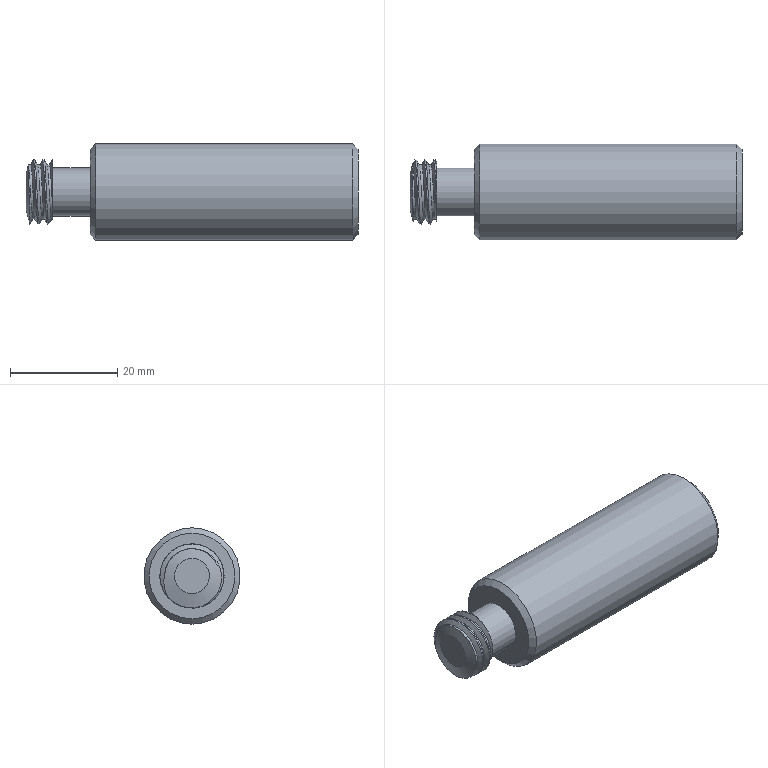Part | NX | features DATUM_CSYS 2, CHAMFER 1, SKETCH 1, SWP104 1, THREADS 1 | 1 solid | 13 faces | box 62 x 18 x 18 mm | volume 13574 mm3 | cylinder 4 | plane 4 | spline 2 | cone 2 | sphere 1 | commonest cylinder face diameters 9 x1 10.25 x1 12 x1 18 x1
STEP:
#1=CARTESIAN_POINT('',(-57.,-2.651,5.382));
#2=VERTEX_POINT('',#1);
#3=CARTESIAN_POINT('',(-57.,2.651,5.382));
#4=VERTEX_POINT('',#3);
#5=CARTESIAN_POINT('',(-57.,0.,0.));
#6=DIRECTION('',(-1.,0.,0.));
#7=DIRECTION('',(0.,0.,1.));
#8=AXIS2_PLACEMENT_3D('',#5,#6,#7);
#9=CIRCLE('',#8,6.);
#10=EDGE_CURVE('',#2,#4,#9,.T.);
#11=ORIENTED_EDGE('',*,*,#10,.T.);
#12=CARTESIAN_POINT('',(-61.271,-0.4952,-5.98));
#13=VERTEX_POINT('',#12);
#14=CARTESIAN_POINT('',(-57.,2.651,5.382));
#15=CARTESIAN_POINT('',(-57.09,4.387,4.527));
#16=CARTESIAN_POINT('',(-57.266,6.894,1.087));
#17=CARTESIAN_POINT('',(-57.534,4.858,-5.032));
#18=CARTESIAN_POINT('',(-57.801,-1.327,-6.864));
#19=CARTESIAN_POINT('',(-58.067,-6.379,-2.86));
#20=CARTESIAN_POINT('',(-58.335,-6.007,3.575));
#21=CARTESIAN_POINT('',(-58.601,-0.5304,6.969));
#22=CARTESIAN_POINT('',(-58.868,5.395,4.444));
#23=CARTESIAN_POINT('',(-59.135,6.739,-1.86));
#24=CARTESIAN_POINT('',(-59.402,2.351,-6.584));
#25=CARTESIAN_POINT('',(-59.669,-4.036,-5.708));
#26=CARTESIAN_POINT('',(-59.936,-6.99,0.02189));
#27=CARTESIAN_POINT('',(-60.203,-4.002,5.73));
#28=CARTESIAN_POINT('',(-60.469,2.383,6.571));
#29=CARTESIAN_POINT('',(-60.736,6.75,1.827));
#30=CARTESIAN_POINT('',(-61.004,5.364,-4.47));
#31=CARTESIAN_POINT('',(-61.18,1.433,-6.139));
#32=CARTESIAN_POINT('',(-61.271,-0.4952,-5.98));
#33=B_SPLINE_CURVE_WITH_KNOTS('',3,(#14,#15,#16,#17,#18,#19,#20,#21,#22,#23,#24,#25,#26,#27,#28,#29,#30,#31,#32),.UNSPECIFIED.,.F.,.F.,(4,1,1,1,1,1,1,1,1,1,1,1,1,1,1,1,4),(0.,0.005728,0.01146,0.01719,0.02291,0.02864,0.03437,0.0401,0.04583,0.05156,0.05728,0.06301,0.06874,0.07447,0.0802,0.08593,0.09165),.UNSPECIFIED.);
#34=EDGE_CURVE('',#4,#13,#33,.T.);
#35=ORIENTED_EDGE('',*,*,#34,.T.);
#36=CARTESIAN_POINT('',(-61.271,4.439,-4.037));
#37=VERTEX_POINT('',#36);
#38=CARTESIAN_POINT('',(-61.271,0.,0.));
#39=DIRECTION('',(-1.,0.,0.));
#40=DIRECTION('',(0.,0.,1.));
#41=AXIS2_PLACEMENT_3D('',#38,#39,#40);
#42=CIRCLE('',#41,6.);
#43=EDGE_CURVE('',#37,#13,#42,.T.);
#44=ORIENTED_EDGE('',*,*,#43,.F.);
#45=CARTESIAN_POINT('',(-61.271,4.439,-4.037));
#46=CARTESIAN_POINT('',(-61.18,5.741,-2.606));
#47=CARTESIAN_POINT('',(-61.004,6.813,1.514));
#48=CARTESIAN_POINT('',(-60.737,2.677,6.462));
#49=CARTESIAN_POINT('',(-60.47,-3.749,5.901));
#50=CARTESIAN_POINT('',(-60.203,-6.983,0.3245));
#51=CARTESIAN_POINT('',(-59.936,-4.279,-5.527));
#52=CARTESIAN_POINT('',(-59.669,2.06,-6.679));
#53=CARTESIAN_POINT('',(-59.402,6.648,-2.158));
#54=CARTESIAN_POINT('',(-59.135,5.589,4.199));
#55=CARTESIAN_POINT('',(-58.869,-0.2242,6.987));
#56=CARTESIAN_POINT('',(-58.601,-5.847,3.832));
#57=CARTESIAN_POINT('',(-58.335,-6.496,-2.581));
#58=CARTESIAN_POINT('',(-58.068,-1.624,-6.798));
#59=CARTESIAN_POINT('',(-57.801,4.625,-5.241));
#60=CARTESIAN_POINT('',(-57.534,6.95,0.7729));
#61=CARTESIAN_POINT('',(-57.267,3.353,6.124));
#62=CARTESIAN_POINT('',(-57.09,-0.9155,6.237));
#63=CARTESIAN_POINT('',(-57.,-2.651,5.382));
#64=B_SPLINE_CURVE_WITH_KNOTS('',3,(#45,#46,#47,#48,#49,#50,#51,#52,#53,#54,#55,#56,#57,#58,#59,#60,#61,#62,#63),.UNSPECIFIED.,.F.,.F.,(4,1,1,1,1,1,1,1,1,1,1,1,1,1,1,1,4),(0.,0.005728,0.01146,0.01719,0.02291,0.02864,0.03437,0.0401,0.04583,0.05156,0.05728,0.06301,0.06874,0.07447,0.0802,0.08593,0.09165),.UNSPECIFIED.);
#65=EDGE_CURVE('',#37,#2,#64,.T.);
#66=ORIENTED_EDGE('',*,*,#65,.T.);
#67=EDGE_LOOP('',(#11,#35,#44,#66));
#68=FACE_BOUND('',#67,.T.);
#69=CARTESIAN_POINT('',(0.,0.,0.));
#70=DIRECTION('',(-1.,0.,0.));
#71=DIRECTION('',(0.,0.,1.));
#72=AXIS2_PLACEMENT_3D('',#69,#70,#71);
#73=CYLINDRICAL_SURFACE('',#72,6.);
#74=ADVANCED_FACE('',(#68),#73,.T.);
#75=CARTESIAN_POINT('',(-62.,0.,3.273));
#76=VERTEX_POINT('',#75);
#77=CARTESIAN_POINT('',(-62.,0.,0.));
#78=DIRECTION('',(-1.,0.,0.));
#79=DIRECTION('',(0.,0.,1.));
#80=AXIS2_PLACEMENT_3D('',#77,#78,#79);
#81=CIRCLE('',#80,3.273);
#82=EDGE_CURVE('',#76,#76,#81,.T.);
#83=ORIENTED_EDGE('',*,*,#82,.F.);
#84=EDGE_LOOP('',(#83));
#85=FACE_BOUND('',#84,.T.);
#86=ORIENTED_EDGE('',*,*,#43,.T.);
#87=CARTESIAN_POINT('',(-61.555,-1.14,4.997));
#88=VERTEX_POINT('',#87);
#89=CARTESIAN_POINT('',(-61.271,-0.4952,-5.98));
#90=CARTESIAN_POINT('',(-61.294,-1.812,-5.804));
#91=CARTESIAN_POINT('',(-61.34,-4.284,-4.566));
#92=CARTESIAN_POINT('',(-61.411,-6.03,-0.7463));
#93=CARTESIAN_POINT('',(-61.483,-4.847,3.306));
#94=CARTESIAN_POINT('',(-61.53,-2.452,4.782));
#95=CARTESIAN_POINT('',(-61.555,-1.14,4.997));
#96=B_SPLINE_CURVE_WITH_KNOTS('',3,(#89,#90,#91,#92,#93,#94,#95),.UNSPECIFIED.,.F.,.F.,(4,1,1,1,4),(0.,0.003931,0.007861,0.01179,0.01572),.UNSPECIFIED.);
#97=EDGE_CURVE('',#13,#88,#96,.T.);
#98=ORIENTED_EDGE('',*,*,#97,.T.);
#99=CARTESIAN_POINT('',(-61.555,5.117,0.2797));
#100=VERTEX_POINT('',#99);
#101=CARTESIAN_POINT('',(-61.555,0.,0.));
#102=DIRECTION('',(1.,0.,0.));
#103=DIRECTION('',(0.,0.,-1.));
#104=AXIS2_PLACEMENT_3D('',#101,#102,#103);
#105=CIRCLE('',#104,5.125);
#106=EDGE_CURVE('',#100,#88,#105,.T.);
#107=ORIENTED_EDGE('',*,*,#106,.F.);
#108=CARTESIAN_POINT('',(-61.555,5.117,0.2797));
#109=CARTESIAN_POINT('',(-61.469,5.486,-1.181));
#110=CARTESIAN_POINT('',(-61.379,5.202,-2.742));
#111=CARTESIAN_POINT('',(-61.271,4.439,-4.037));
#112=B_SPLINE_CURVE_WITH_KNOTS('',3,(#108,#109,#110,#111),.UNSPECIFIED.,.F.,.F.,(4,4),(0.00002886,0.004494),.UNSPECIFIED.);
#113=EDGE_CURVE('',#100,#37,#112,.T.);
#114=ORIENTED_EDGE('',*,*,#113,.T.);
#115=EDGE_LOOP('',(#86,#98,#107,#114));
#116=FACE_BOUND('',#115,.T.);
#117=CARTESIAN_POINT('',(-44.3,0.,0.));
#118=DIRECTION('',(-1.,0.,0.));
#119=DIRECTION('',(0.,1.,0.));
#120=AXIS2_PLACEMENT_3D('',#117,#118,#119);
#121=SPHERICAL_SURFACE('',#120,18.);
#122=ADVANCED_FACE('',(#85,#116),#121,.T.);
#123=ORIENTED_EDGE('',*,*,#82,.T.);
#124=EDGE_LOOP('',(#123));
#125=FACE_BOUND('',#124,.T.);
#126=CARTESIAN_POINT('',(-62.,3.273,0.));
#127=DIRECTION('',(1.,0.,0.));
#128=DIRECTION('',(0.,0.,-1.));
#129=AXIS2_PLACEMENT_3D('',#126,#127,#128);
#130=PLANE('',#129);
#131=ADVANCED_FACE('',(#125),#130,.F.);
#132=CARTESIAN_POINT('',(0.,0.,8.));
#133=VERTEX_POINT('',#132);
#134=CARTESIAN_POINT('',(0.,0.,0.));
#135=DIRECTION('',(-1.,0.,0.));
#136=DIRECTION('',(0.,0.,1.));
#137=AXIS2_PLACEMENT_3D('',#134,#135,#136);
#138=CIRCLE('',#137,8.);
#139=EDGE_CURVE('',#133,#133,#138,.F.);
#140=ORIENTED_EDGE('',*,*,#139,.T.);
#141=EDGE_LOOP('',(#140));
#142=FACE_BOUND('',#141,.T.);
#143=CARTESIAN_POINT('',(0.,0.,0.));
#144=DIRECTION('',(-1.,0.,0.));
#145=DIRECTION('',(0.,0.,1.));
#146=AXIS2_PLACEMENT_3D('',#143,#144,#145);
#147=PLANE('',#146);
#148=ADVANCED_FACE('',(#142),#147,.F.);
#149=CARTESIAN_POINT('',(-49.,0.,-9.));
#150=VERTEX_POINT('',#149);
#151=CARTESIAN_POINT('',(-49.,0.,0.));
#152=DIRECTION('',(1.,0.,0.));
#153=DIRECTION('',(0.,0.,-1.));
#154=AXIS2_PLACEMENT_3D('',#151,#152,#153);
#155=CIRCLE('',#154,9.);
#156=EDGE_CURVE('',#150,#150,#155,.T.);
#157=ORIENTED_EDGE('',*,*,#156,.T.);
#158=EDGE_LOOP('',(#157));
#159=FACE_BOUND('',#158,.T.);
#160=CARTESIAN_POINT('',(-1.,0.,9.));
#161=VERTEX_POINT('',#160);
#162=CARTESIAN_POINT('',(-1.,0.,0.));
#163=DIRECTION('',(-1.,0.,0.));
#164=DIRECTION('',(0.,0.,1.));
#165=AXIS2_PLACEMENT_3D('',#162,#163,#164);
#166=CIRCLE('',#165,9.);
#167=EDGE_CURVE('',#161,#161,#166,.T.);
#168=ORIENTED_EDGE('',*,*,#167,.T.);
#169=EDGE_LOOP('',(#168));
#170=FACE_BOUND('',#169,.T.);
#171=CARTESIAN_POINT('',(0.,0.,0.));
#172=DIRECTION('',(-1.,0.,0.));
#173=DIRECTION('',(0.,0.,1.));
#174=AXIS2_PLACEMENT_3D('',#171,#172,#173);
#175=CYLINDRICAL_SURFACE('',#174,9.);
#176=ADVANCED_FACE('',(#159,#170),#175,.T.);
#177=CARTESIAN_POINT('',(-50.,0.,-8.));
#178=VERTEX_POINT('',#177);
#179=CARTESIAN_POINT('',(-50.,0.,0.));
#180=DIRECTION('',(1.,0.,0.));
#181=DIRECTION('',(0.,0.,-1.));
#182=AXIS2_PLACEMENT_3D('',#179,#180,#181);
#183=CIRCLE('',#182,8.);
#184=EDGE_CURVE('',#178,#178,#183,.F.);
#185=ORIENTED_EDGE('',*,*,#184,.T.);
#186=EDGE_LOOP('',(#185));
#187=FACE_BOUND('',#186,.T.);
#188=CARTESIAN_POINT('',(-50.,0.,4.5));
#189=VERTEX_POINT('',#188);
#190=CARTESIAN_POINT('',(-50.,0.,0.));
#191=DIRECTION('',(-1.,0.,0.));
#192=DIRECTION('',(0.,0.,1.));
#193=AXIS2_PLACEMENT_3D('',#190,#191,#192);
#194=CIRCLE('',#193,4.5);
#195=EDGE_CURVE('',#189,#189,#194,.T.);
#196=ORIENTED_EDGE('',*,*,#195,.F.);
#197=EDGE_LOOP('',(#196));
#198=FACE_BOUND('',#197,.T.);
#199=CARTESIAN_POINT('',(-50.,9.,0.));
#200=DIRECTION('',(1.,0.,0.));
#201=DIRECTION('',(0.,0.,-1.));
#202=AXIS2_PLACEMENT_3D('',#199,#200,#201);
#203=PLANE('',#202);
#204=ADVANCED_FACE('',(#187,#198),#203,.F.);
#205=CARTESIAN_POINT('',(-57.,0.,4.5));
#206=VERTEX_POINT('',#205);
#207=CARTESIAN_POINT('',(-57.,0.,0.));
#208=DIRECTION('',(-1.,0.,0.));
#209=DIRECTION('',(0.,0.,1.));
#210=AXIS2_PLACEMENT_3D('',#207,#208,#209);
#211=CIRCLE('',#210,4.5);
#212=EDGE_CURVE('',#206,#206,#211,.T.);
#213=ORIENTED_EDGE('',*,*,#212,.F.);
#214=EDGE_LOOP('',(#213));
#215=FACE_BOUND('',#214,.T.);
#216=ORIENTED_EDGE('',*,*,#195,.T.);
#217=EDGE_LOOP('',(#216));
#218=FACE_BOUND('',#217,.T.);
#219=CARTESIAN_POINT('',(0.,0.,0.));
#220=DIRECTION('',(-1.,0.,0.));
#221=DIRECTION('',(0.,0.,1.));
#222=AXIS2_PLACEMENT_3D('',#219,#220,#221);
#223=CYLINDRICAL_SURFACE('',#222,4.5);
#224=ADVANCED_FACE('',(#215,#218),#223,.T.);
#225=ORIENTED_EDGE('',*,*,#10,.F.);
#226=CARTESIAN_POINT('',(-57.,-3.918,-3.304));
#227=VERTEX_POINT('',#226);
#228=CARTESIAN_POINT('',(-57.,-2.651,5.382));
#229=CARTESIAN_POINT('',(-57.,-4.109,4.512));
#230=CARTESIAN_POINT('',(-57.,-6.212,1.478));
#231=CARTESIAN_POINT('',(-57.,-5.133,-2.11));
#232=CARTESIAN_POINT('',(-57.,-3.918,-3.304));
#233=B_SPLINE_CURVE_WITH_KNOTS('',3,(#228,#229,#230,#231,#232),.UNSPECIFIED.,.F.,.F.,(4,1,4),(0.0001216,0.005159,0.0102),.UNSPECIFIED.);
#234=EDGE_CURVE('',#2,#227,#233,.T.);
#235=ORIENTED_EDGE('',*,*,#234,.T.);
#236=CARTESIAN_POINT('',(-57.,3.918,-3.304));
#237=VERTEX_POINT('',#236);
#238=CARTESIAN_POINT('',(-57.,0.,0.));
#239=DIRECTION('',(-1.,0.,0.));
#240=DIRECTION('',(0.,0.,1.));
#241=AXIS2_PLACEMENT_3D('',#238,#239,#240);
#242=CIRCLE('',#241,5.125);
#243=EDGE_CURVE('',#237,#227,#242,.T.);
#244=ORIENTED_EDGE('',*,*,#243,.F.);
#245=CARTESIAN_POINT('',(-57.,3.918,-3.304));
#246=CARTESIAN_POINT('',(-57.,5.13,-2.112));
#247=CARTESIAN_POINT('',(-57.,6.216,1.465));
#248=CARTESIAN_POINT('',(-57.,4.109,4.512));
#249=CARTESIAN_POINT('',(-57.,2.651,5.382));
#250=B_SPLINE_CURVE_WITH_KNOTS('',3,(#245,#246,#247,#248,#249),.UNSPECIFIED.,.F.,.F.,(4,1,4),(0.00005946,0.005098,0.01014),.UNSPECIFIED.);
#251=EDGE_CURVE('',#237,#4,#250,.T.);
#252=ORIENTED_EDGE('',*,*,#251,.T.);
#253=EDGE_LOOP('',(#225,#235,#244,#252));
#254=FACE_BOUND('',#253,.T.);
#255=ORIENTED_EDGE('',*,*,#212,.T.);
#256=EDGE_LOOP('',(#255));
#257=FACE_BOUND('',#256,.T.);
#258=CARTESIAN_POINT('',(-57.,4.5,0.));
#259=DIRECTION('',(-1.,0.,0.));
#260=DIRECTION('',(0.,0.,1.));
#261=AXIS2_PLACEMENT_3D('',#258,#259,#260);
#262=PLANE('',#261);
#263=ADVANCED_FACE('',(#254,#257),#262,.F.);
#264=ORIENTED_EDGE('',*,*,#243,.T.);
#265=CARTESIAN_POINT('',(-61.555,5.117,0.2797));
#266=CARTESIAN_POINT('',(-61.46,5.022,2.017));
#267=CARTESIAN_POINT('',(-61.27,2.892,5.365));
#268=CARTESIAN_POINT('',(-60.985,-3.072,5.268));
#269=CARTESIAN_POINT('',(-60.701,-6.096,0.1263));
#270=CARTESIAN_POINT('',(-60.416,-3.288,-5.135));
#271=CARTESIAN_POINT('',(-60.132,2.667,-5.483));
#272=CARTESIAN_POINT('',(-59.847,6.069,-0.5848));
#273=CARTESIAN_POINT('',(-59.562,3.664,4.873));
#274=CARTESIAN_POINT('',(-59.278,-2.247,5.668));
#275=CARTESIAN_POINT('',(-58.993,-6.008,1.039));
#276=CARTESIAN_POINT('',(-58.708,-4.02,-4.584));
#277=CARTESIAN_POINT('',(-58.423,1.815,-5.821));
#278=CARTESIAN_POINT('',(-58.139,5.913,-1.487));
#279=CARTESIAN_POINT('',(-57.854,4.354,4.269));
#280=CARTESIAN_POINT('',(-57.569,-1.375,5.943));
#281=CARTESIAN_POINT('',(-57.285,-5.778,1.919));
#282=CARTESIAN_POINT('',(-57.095,-5.05,-1.961));
#283=CARTESIAN_POINT('',(-57.,-3.918,-3.304));
#284=B_SPLINE_CURVE_WITH_KNOTS('',3,(#265,#266,#267,#268,#269,#270,#271,#272,#273,#274,#275,#276,#277,#278,#279,#280,#281,#282,#283),.UNSPECIFIED.,.F.,.F.,(4,1,1,1,1,1,1,1,1,1,1,1,1,1,1,1,4),(0.009769,0.01499,0.02021,0.02543,0.03065,0.03588,0.0411,0.04632,0.05154,0.05676,0.06198,0.0672,0.07242,0.07764,0.08287,0.08809,0.09331),.UNSPECIFIED.);
#285=EDGE_CURVE('',#227,#100,#284,.F.);
#286=ORIENTED_EDGE('',*,*,#285,.T.);
#287=ORIENTED_EDGE('',*,*,#106,.T.);
#288=CARTESIAN_POINT('',(-57.,3.918,-3.304));
#289=CARTESIAN_POINT('',(-57.094,2.794,-4.636));
#290=CARTESIAN_POINT('',(-57.285,-0.9202,-6.024));
#291=CARTESIAN_POINT('',(-57.569,-5.624,-2.357));
#292=CARTESIAN_POINT('',(-57.854,-4.944,3.569));
#293=CARTESIAN_POINT('',(-58.139,0.4663,6.079));
#294=CARTESIAN_POINT('',(-58.423,5.43,2.773));
#295=CARTESIAN_POINT('',(-58.708,5.198,-3.187));
#296=CARTESIAN_POINT('',(-58.992,-0.00777,-6.097));
#297=CARTESIAN_POINT('',(-59.278,-5.206,-3.174));
#298=CARTESIAN_POINT('',(-59.562,-5.423,2.787));
#299=CARTESIAN_POINT('',(-59.847,-0.4504,6.081));
#300=CARTESIAN_POINT('',(-60.132,4.954,3.556));
#301=CARTESIAN_POINT('',(-60.416,5.617,-2.372));
#302=CARTESIAN_POINT('',(-60.701,0.9062,-6.03));
#303=CARTESIAN_POINT('',(-60.985,-4.675,-3.918));
#304=CARTESIAN_POINT('',(-61.27,-5.771,1.945));
#305=CARTESIAN_POINT('',(-61.46,-2.848,4.607));
#306=CARTESIAN_POINT('',(-61.555,-1.14,4.997));
#307=B_SPLINE_CURVE_WITH_KNOTS('',3,(#288,#289,#290,#291,#292,#293,#294,#295,#296,#297,#298,#299,#300,#301,#302,#303,#304,#305,#306),.UNSPECIFIED.,.F.,.F.,(4,1,1,1,1,1,1,1,1,1,1,1,1,1,1,1,4),(0.0116,0.01683,0.02205,0.02727,0.03249,0.03771,0.04293,0.04815,0.05337,0.05859,0.06382,0.06904,0.07426,0.07948,0.0847,0.08992,0.09514),.UNSPECIFIED.);
#308=EDGE_CURVE('',#88,#237,#307,.F.);
#309=ORIENTED_EDGE('',*,*,#308,.T.);
#310=EDGE_LOOP('',(#264,#286,#287,#309));
#311=FACE_BOUND('',#310,.T.);
#312=CARTESIAN_POINT('',(-56.125,0.,0.));
#313=DIRECTION('',(-1.,0.,0.));
#314=DIRECTION('',(0.,0.,1.));
#315=AXIS2_PLACEMENT_3D('',#312,#313,#314);
#316=CYLINDRICAL_SURFACE('',#315,5.125);
#317=ADVANCED_FACE('',(#311),#316,.T.);
#318=ORIENTED_EDGE('',*,*,#308,.F.);
#319=ORIENTED_EDGE('',*,*,#97,.F.);
#320=ORIENTED_EDGE('',*,*,#34,.F.);
#321=ORIENTED_EDGE('',*,*,#251,.F.);
#322=EDGE_LOOP('',(#318,#319,#320,#321));
#323=FACE_BOUND('',#322,.T.);
#324=CARTESIAN_POINT('',(-56.461,1.749,4.811));
#325=CARTESIAN_POINT('',(-56.465,1.82,4.786));
#326=CARTESIAN_POINT('',(-56.506,2.515,4.516));
#327=CARTESIAN_POINT('',(-56.583,3.714,3.714));
#328=CARTESIAN_POINT('',(-56.692,4.853,2.01));
#329=CARTESIAN_POINT('',(-56.802,5.253,0.));
#330=CARTESIAN_POINT('',(-56.911,4.853,-2.01));
#331=CARTESIAN_POINT('',(-57.02,3.714,-3.714));
#332=CARTESIAN_POINT('',(-57.13,2.01,-4.853));
#333=CARTESIAN_POINT('',(-57.239,0.,-5.253));
#334=CARTESIAN_POINT('',(-57.348,-2.01,-4.853));
#335=CARTESIAN_POINT('',(-57.458,-3.714,-3.714));
#336=CARTESIAN_POINT('',(-57.567,-4.853,-2.01));
#337=CARTESIAN_POINT('',(-57.677,-5.253,0.));
#338=CARTESIAN_POINT('',(-57.786,-4.853,2.01));
#339=CARTESIAN_POINT('',(-57.895,-3.714,3.714));
#340=CARTESIAN_POINT('',(-58.005,-2.01,4.853));
#341=CARTESIAN_POINT('',(-58.114,0.,5.253));
#342=CARTESIAN_POINT('',(-58.223,2.01,4.853));
#343=CARTESIAN_POINT('',(-58.333,3.714,3.714));
#344=CARTESIAN_POINT('',(-58.442,4.853,2.01));
#345=CARTESIAN_POINT('',(-58.552,5.253,0.));
#346=CARTESIAN_POINT('',(-58.661,4.853,-2.01));
#347=CARTESIAN_POINT('',(-58.77,3.714,-3.714));
#348=CARTESIAN_POINT('',(-58.88,2.01,-4.853));
#349=CARTESIAN_POINT('',(-58.989,0.,-5.253));
#350=CARTESIAN_POINT('',(-59.098,-2.01,-4.853));
#351=CARTESIAN_POINT('',(-59.208,-3.714,-3.714));
#352=CARTESIAN_POINT('',(-59.317,-4.853,-2.01));
#353=CARTESIAN_POINT('',(-59.427,-5.253,0.));
#354=CARTESIAN_POINT('',(-59.536,-4.853,2.01));
#355=CARTESIAN_POINT('',(-59.645,-3.714,3.714));
#356=CARTESIAN_POINT('',(-59.755,-2.01,4.853));
#357=CARTESIAN_POINT('',(-59.864,0.,5.253));
#358=CARTESIAN_POINT('',(-59.973,2.01,4.853));
#359=CARTESIAN_POINT('',(-60.083,3.714,3.714));
#360=CARTESIAN_POINT('',(-60.192,4.853,2.01));
#361=CARTESIAN_POINT('',(-60.302,5.253,0.));
#362=CARTESIAN_POINT('',(-60.411,4.853,-2.01));
#363=CARTESIAN_POINT('',(-60.52,3.714,-3.714));
#364=CARTESIAN_POINT('',(-60.63,2.01,-4.853));
#365=CARTESIAN_POINT('',(-60.739,0.,-5.253));
#366=CARTESIAN_POINT('',(-60.848,-2.01,-4.853));
#367=CARTESIAN_POINT('',(-60.958,-3.714,-3.714));
#368=CARTESIAN_POINT('',(-61.067,-4.853,-2.01));
#369=CARTESIAN_POINT('',(-61.177,-5.253,0.));
#370=CARTESIAN_POINT('',(-61.286,-4.853,2.01));
#371=CARTESIAN_POINT('',(-61.395,-3.714,3.714));
#372=CARTESIAN_POINT('',(-61.494,-2.177,4.742));
#373=CARTESIAN_POINT('',(-61.556,-1.059,5.031));
#374=CARTESIAN_POINT('',(-61.582,-0.5889,5.085));
#375=CARTESIAN_POINT('',(-56.973,2.052,5.644));
#376=CARTESIAN_POINT('',(-56.977,2.135,5.614));
#377=CARTESIAN_POINT('',(-57.018,2.95,5.298));
#378=CARTESIAN_POINT('',(-57.095,4.357,4.357));
#379=CARTESIAN_POINT('',(-57.204,5.693,2.358));
#380=CARTESIAN_POINT('',(-57.313,6.162,0.));
#381=CARTESIAN_POINT('',(-57.423,5.693,-2.358));
#382=CARTESIAN_POINT('',(-57.532,4.357,-4.357));
#383=CARTESIAN_POINT('',(-57.641,2.358,-5.693));
#384=CARTESIAN_POINT('',(-57.751,0.,-6.162));
#385=CARTESIAN_POINT('',(-57.86,-2.358,-5.693));
#386=CARTESIAN_POINT('',(-57.97,-4.357,-4.357));
#387=CARTESIAN_POINT('',(-58.079,-5.693,-2.358));
#388=CARTESIAN_POINT('',(-58.188,-6.162,0.));
#389=CARTESIAN_POINT('',(-58.298,-5.693,2.358));
#390=CARTESIAN_POINT('',(-58.407,-4.357,4.357));
#391=CARTESIAN_POINT('',(-58.516,-2.358,5.693));
#392=CARTESIAN_POINT('',(-58.626,0.,6.162));
#393=CARTESIAN_POINT('',(-58.735,2.358,5.693));
#394=CARTESIAN_POINT('',(-58.845,4.357,4.357));
#395=CARTESIAN_POINT('',(-58.954,5.693,2.358));
#396=CARTESIAN_POINT('',(-59.063,6.162,0.));
#397=CARTESIAN_POINT('',(-59.173,5.693,-2.358));
#398=CARTESIAN_POINT('',(-59.282,4.357,-4.357));
#399=CARTESIAN_POINT('',(-59.391,2.358,-5.693));
#400=CARTESIAN_POINT('',(-59.501,0.,-6.162));
#401=CARTESIAN_POINT('',(-59.61,-2.358,-5.693));
#402=CARTESIAN_POINT('',(-59.72,-4.357,-4.357));
#403=CARTESIAN_POINT('',(-59.829,-5.693,-2.358));
#404=CARTESIAN_POINT('',(-59.938,-6.162,0.));
#405=CARTESIAN_POINT('',(-60.048,-5.693,2.358));
#406=CARTESIAN_POINT('',(-60.157,-4.357,4.357));
#407=CARTESIAN_POINT('',(-60.266,-2.358,5.693));
#408=CARTESIAN_POINT('',(-60.376,0.,6.162));
#409=CARTESIAN_POINT('',(-60.485,2.358,5.693));
#410=CARTESIAN_POINT('',(-60.595,4.357,4.357));
#411=CARTESIAN_POINT('',(-60.704,5.693,2.358));
#412=CARTESIAN_POINT('',(-60.813,6.162,0.));
#413=CARTESIAN_POINT('',(-60.923,5.693,-2.358));
#414=CARTESIAN_POINT('',(-61.032,4.357,-4.357));
#415=CARTESIAN_POINT('',(-61.141,2.358,-5.693));
#416=CARTESIAN_POINT('',(-61.251,0.,-6.162));
#417=CARTESIAN_POINT('',(-61.36,-2.358,-5.693));
#418=CARTESIAN_POINT('',(-61.47,-4.357,-4.357));
#419=CARTESIAN_POINT('',(-61.579,-5.693,-2.358));
#420=CARTESIAN_POINT('',(-61.688,-6.162,0.));
#421=CARTESIAN_POINT('',(-61.798,-5.693,2.358));
#422=CARTESIAN_POINT('',(-61.907,-4.357,4.357));
#423=CARTESIAN_POINT('',(-62.006,-2.554,5.562));
#424=CARTESIAN_POINT('',(-62.068,-1.242,5.902));
#425=CARTESIAN_POINT('',(-62.094,-0.6909,5.966));
#426=B_SPLINE_SURFACE_WITH_KNOTS('',1,3,((#324,#325,#326,#327,#328,#329,#330,#331,#332,#333,#334,#335,#336,#337,#338,#339,#340,#341,#342,#343,#344,#345,#346,#347,#348,#349,#350,#351,#352,#353,#354,#355,#356,#357,#358,#359,#360,#361,#362,#363,#364,#365,#366,#367,#368,#369,#370,#371,#372,#373,#374),(#375,#376,#377,#378,#379,#380,#381,#382,#383,#384,#385,#386,#387,#388,#389,#390,#391,#392,#393,#394,#395,#396,#397,#398,#399,#400,#401,#402,#403,#404,#405,#406,#407,#408,#409,#410,#411,#412,#413,#414,#415,#416,#417,#418,#419,#420,#421,#422,#423,#424,#425)),.RULED_SURF.,.F.,.F.,.F.,(2,2),(4,1,1,1,1,1,1,1,1,1,1,1,1,1,1,1,1,1,1,1,1,1,1,1,1,1,1,1,1,1,1,1,1,1,1,1,1,1,1,1,1,1,1,1,1,1,1,1,4),(0.241,0.9965),(0.01565,0.01763,0.03525,0.05288,0.07051,0.08814,0.1058,0.1234,0.141,0.1586,0.1763,0.1939,0.2115,0.2292,0.2468,0.2644,0.282,0.2997,0.3173,0.3349,0.3525,0.3702,0.3878,0.4054,0.4231,0.4407,0.4583,0.4759,0.4936,0.5112,0.5288,0.5464,0.5641,0.5817,0.5993,0.617,0.6346,0.6522,0.6698,0.6875,0.7051,0.7227,0.7403,0.758,0.7756,0.7932,0.8109,0.8285,0.8409),.UNSPECIFIED.);
#427=ADVANCED_FACE('',(#323),#426,.F.);
#428=ORIENTED_EDGE('',*,*,#65,.F.);
#429=ORIENTED_EDGE('',*,*,#113,.F.);
#430=ORIENTED_EDGE('',*,*,#285,.F.);
#431=ORIENTED_EDGE('',*,*,#234,.F.);
#432=EDGE_LOOP('',(#428,#429,#430,#431));
#433=FACE_BOUND('',#432,.T.);
#434=CARTESIAN_POINT('',(-56.463,-4.169,-4.323));
#435=CARTESIAN_POINT('',(-56.465,-4.195,-4.298));
#436=CARTESIAN_POINT('',(-56.503,-4.782,-3.722));
#437=CARTESIAN_POINT('',(-56.577,-5.693,-2.358));
#438=CARTESIAN_POINT('',(-56.687,-6.162,0.));
#439=CARTESIAN_POINT('',(-56.796,-5.693,2.358));
#440=CARTESIAN_POINT('',(-56.905,-4.357,4.357));
#441=CARTESIAN_POINT('',(-57.015,-2.358,5.693));
#442=CARTESIAN_POINT('',(-57.124,0.,6.162));
#443=CARTESIAN_POINT('',(-57.234,2.358,5.693));
#444=CARTESIAN_POINT('',(-57.343,4.357,4.357));
#445=CARTESIAN_POINT('',(-57.452,5.693,2.358));
#446=CARTESIAN_POINT('',(-57.562,6.162,0.));
#447=CARTESIAN_POINT('',(-57.671,5.693,-2.358));
#448=CARTESIAN_POINT('',(-57.78,4.357,-4.357));
#449=CARTESIAN_POINT('',(-57.89,2.358,-5.693));
#450=CARTESIAN_POINT('',(-57.999,0.,-6.162));
#451=CARTESIAN_POINT('',(-58.109,-2.358,-5.693));
#452=CARTESIAN_POINT('',(-58.218,-4.357,-4.357));
#453=CARTESIAN_POINT('',(-58.327,-5.693,-2.358));
#454=CARTESIAN_POINT('',(-58.437,-6.162,0.));
#455=CARTESIAN_POINT('',(-58.546,-5.693,2.358));
#456=CARTESIAN_POINT('',(-58.655,-4.357,4.357));
#457=CARTESIAN_POINT('',(-58.765,-2.358,5.693));
#458=CARTESIAN_POINT('',(-58.874,0.,6.162));
#459=CARTESIAN_POINT('',(-58.984,2.358,5.693));
#460=CARTESIAN_POINT('',(-59.093,4.357,4.357));
#461=CARTESIAN_POINT('',(-59.202,5.693,2.358));
#462=CARTESIAN_POINT('',(-59.312,6.162,0.));
#463=CARTESIAN_POINT('',(-59.421,5.693,-2.358));
#464=CARTESIAN_POINT('',(-59.53,4.357,-4.357));
#465=CARTESIAN_POINT('',(-59.64,2.358,-5.693));
#466=CARTESIAN_POINT('',(-59.749,0.,-6.162));
#467=CARTESIAN_POINT('',(-59.859,-2.358,-5.693));
#468=CARTESIAN_POINT('',(-59.968,-4.357,-4.357));
#469=CARTESIAN_POINT('',(-60.077,-5.693,-2.358));
#470=CARTESIAN_POINT('',(-60.187,-6.162,0.));
#471=CARTESIAN_POINT('',(-60.296,-5.693,2.358));
#472=CARTESIAN_POINT('',(-60.405,-4.357,4.357));
#473=CARTESIAN_POINT('',(-60.515,-2.358,5.693));
#474=CARTESIAN_POINT('',(-60.624,0.,6.162));
#475=CARTESIAN_POINT('',(-60.734,2.358,5.693));
#476=CARTESIAN_POINT('',(-60.843,4.357,4.357));
#477=CARTESIAN_POINT('',(-60.952,5.693,2.358));
#478=CARTESIAN_POINT('',(-61.062,6.162,0.));
#479=CARTESIAN_POINT('',(-61.171,5.693,-2.358));
#480=CARTESIAN_POINT('',(-61.249,4.74,-3.785));
#481=CARTESIAN_POINT('',(-61.291,4.087,-4.402));
#482=CARTESIAN_POINT('',(-61.296,4.005,-4.476));
#483=CARTESIAN_POINT('',(-56.975,-3.554,-3.685));
#484=CARTESIAN_POINT('',(-56.976,-3.576,-3.664));
#485=CARTESIAN_POINT('',(-57.014,-4.076,-3.173));
#486=CARTESIAN_POINT('',(-57.089,-4.853,-2.01));
#487=CARTESIAN_POINT('',(-57.198,-5.253,0.));
#488=CARTESIAN_POINT('',(-57.308,-4.853,2.01));
#489=CARTESIAN_POINT('',(-57.417,-3.714,3.714));
#490=CARTESIAN_POINT('',(-57.527,-2.01,4.853));
#491=CARTESIAN_POINT('',(-57.636,0.,5.253));
#492=CARTESIAN_POINT('',(-57.745,2.01,4.853));
#493=CARTESIAN_POINT('',(-57.855,3.714,3.714));
#494=CARTESIAN_POINT('',(-57.964,4.853,2.01));
#495=CARTESIAN_POINT('',(-58.073,5.253,0.));
#496=CARTESIAN_POINT('',(-58.183,4.853,-2.01));
#497=CARTESIAN_POINT('',(-58.292,3.714,-3.714));
#498=CARTESIAN_POINT('',(-58.402,2.01,-4.853));
#499=CARTESIAN_POINT('',(-58.511,0.,-5.253));
#500=CARTESIAN_POINT('',(-58.62,-2.01,-4.853));
#501=CARTESIAN_POINT('',(-58.73,-3.714,-3.714));
#502=CARTESIAN_POINT('',(-58.839,-4.853,-2.01));
#503=CARTESIAN_POINT('',(-58.948,-5.253,0.));
#504=CARTESIAN_POINT('',(-59.058,-4.853,2.01));
#505=CARTESIAN_POINT('',(-59.167,-3.714,3.714));
#506=CARTESIAN_POINT('',(-59.277,-2.01,4.853));
#507=CARTESIAN_POINT('',(-59.386,0.,5.253));
#508=CARTESIAN_POINT('',(-59.495,2.01,4.853));
#509=CARTESIAN_POINT('',(-59.605,3.714,3.714));
#510=CARTESIAN_POINT('',(-59.714,4.853,2.01));
#511=CARTESIAN_POINT('',(-59.823,5.253,0.));
#512=CARTESIAN_POINT('',(-59.933,4.853,-2.01));
#513=CARTESIAN_POINT('',(-60.042,3.714,-3.714));
#514=CARTESIAN_POINT('',(-60.152,2.01,-4.853));
#515=CARTESIAN_POINT('',(-60.261,0.,-5.253));
#516=CARTESIAN_POINT('',(-60.37,-2.01,-4.853));
#517=CARTESIAN_POINT('',(-60.48,-3.714,-3.714));
#518=CARTESIAN_POINT('',(-60.589,-4.853,-2.01));
#519=CARTESIAN_POINT('',(-60.698,-5.253,0.));
#520=CARTESIAN_POINT('',(-60.808,-4.853,2.01));
#521=CARTESIAN_POINT('',(-60.917,-3.714,3.714));
#522=CARTESIAN_POINT('',(-61.027,-2.01,4.853));
#523=CARTESIAN_POINT('',(-61.136,0.,5.253));
#524=CARTESIAN_POINT('',(-61.245,2.01,4.853));
#525=CARTESIAN_POINT('',(-61.355,3.714,3.714));
#526=CARTESIAN_POINT('',(-61.464,4.853,2.01));
#527=CARTESIAN_POINT('',(-61.573,5.253,0.));
#528=CARTESIAN_POINT('',(-61.683,4.853,-2.01));
#529=CARTESIAN_POINT('',(-61.761,4.04,-3.227));
#530=CARTESIAN_POINT('',(-61.802,3.484,-3.752));
#531=CARTESIAN_POINT('',(-61.808,3.414,-3.815));
#532=B_SPLINE_SURFACE_WITH_KNOTS('',1,3,((#434,#435,#436,#437,#438,#439,#440,#441,#442,#443,#444,#445,#446,#447,#448,#449,#450,#451,#452,#453,#454,#455,#456,#457,#458,#459,#460,#461,#462,#463,#464,#465,#466,#467,#468,#469,#470,#471,#472,#473,#474,#475,#476,#477,#478,#479,#480,#481,#482),(#483,#484,#485,#486,#487,#488,#489,#490,#491,#492,#493,#494,#495,#496,#497,#498,#499,#500,#501,#502,#503,#504,#505,#506,#507,#508,#509,#510,#511,#512,#513,#514,#515,#516,#517,#518,#519,#520,#521,#522,#523,#524,#525,#526,#527,#528,#529,#530,#531)),.RULED_SURF.,.F.,.F.,.F.,(2,2),(4,1,1,1,1,1,1,1,1,1,1,1,1,1,1,1,1,1,1,1,1,1,1,1,1,1,1,1,1,1,1,1,1,1,1,1,1,1,1,1,1,1,1,1,1,1,4),(0.003551,0.759),(0.1755,0.1763,0.1939,0.2115,0.2292,0.2468,0.2644,0.282,0.2997,0.3173,0.3349,0.3525,0.3702,0.3878,0.4054,0.4231,0.4407,0.4583,0.4759,0.4936,0.5112,0.5288,0.5464,0.5641,0.5817,0.5993,0.617,0.6346,0.6522,0.6698,0.6875,0.7051,0.7227,0.7403,0.758,0.7756,0.7932,0.8109,0.8285,0.8461,0.8637,0.8814,0.899,0.9166,0.9342,0.9519,0.9544),.UNSPECIFIED.);
#533=ADVANCED_FACE('',(#433),#532,.F.);
#534=ORIENTED_EDGE('',*,*,#156,.F.);
#535=EDGE_LOOP('',(#534));
#536=FACE_BOUND('',#535,.T.);
#537=ORIENTED_EDGE('',*,*,#184,.F.);
#538=EDGE_LOOP('',(#537));
#539=FACE_BOUND('',#538,.T.);
#540=CARTESIAN_POINT('',(-50.,0.,0.));
#541=DIRECTION('',(1.,0.,0.));
#542=DIRECTION('',(0.,0.,-1.));
#543=AXIS2_PLACEMENT_3D('',#540,#541,#542);
#544=CONICAL_SURFACE('',#543,8.,0.7854);
#545=ADVANCED_FACE('',(#536,#539),#544,.T.);
#546=ORIENTED_EDGE('',*,*,#139,.F.);
#547=EDGE_LOOP('',(#546));
#548=FACE_BOUND('',#547,.T.);
#549=ORIENTED_EDGE('',*,*,#167,.F.);
#550=EDGE_LOOP('',(#549));
#551=FACE_BOUND('',#550,.T.);
#552=CARTESIAN_POINT('',(-1.,0.,0.));
#553=DIRECTION('',(-1.,0.,0.));
#554=DIRECTION('',(0.,0.,1.));
#555=AXIS2_PLACEMENT_3D('',#552,#553,#554);
#556=CONICAL_SURFACE('',#555,9.,0.7854);
#557=ADVANCED_FACE('',(#548,#551),#556,.T.);
#558=CLOSED_SHELL('',(#74,#122,#131,#148,#176,#204,#224,#263,#317,#427,#533,#545,#557));
#559=MANIFOLD_SOLID_BREP('',#558);
#560=(LENGTH_UNIT()NAMED_UNIT(*)SI_UNIT(.MILLI.,.METRE.));
#561=UNCERTAINTY_MEASURE_WITH_UNIT(LENGTH_MEASURE(0.0508),#560,'','');
#562=(NAMED_UNIT(*)PLANE_ANGLE_UNIT()SI_UNIT($,.RADIAN.));
#563=(NAMED_UNIT(*)SI_UNIT($,.STERADIAN.)SOLID_ANGLE_UNIT());
#564=(GEOMETRIC_REPRESENTATION_CONTEXT(3)GLOBAL_UNCERTAINTY_ASSIGNED_CONTEXT((#561))GLOBAL_UNIT_ASSIGNED_CONTEXT((#560,#562,#563))REPRESENTATION_CONTEXT('',''));
#565=ADVANCED_BREP_SHAPE_REPRESENTATION('',(#559),#564);